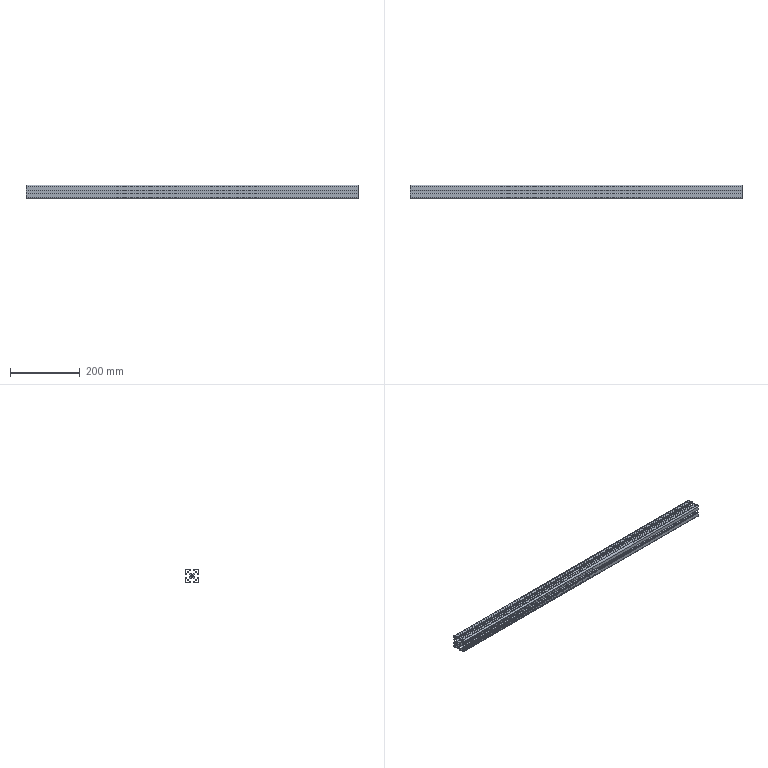Part | STEP file | MK-8-4040C-L-00 profile 4040C standard 950mm | 1 solid | 188 faces | box 950 x 40 x 40 mm | volume 454336 mm3 | cylinder 94 | plane 94 | commonest cylinder face diameters 0.6 x30 2 x28 4 x16 0.4 x8 6 x4 9 x4